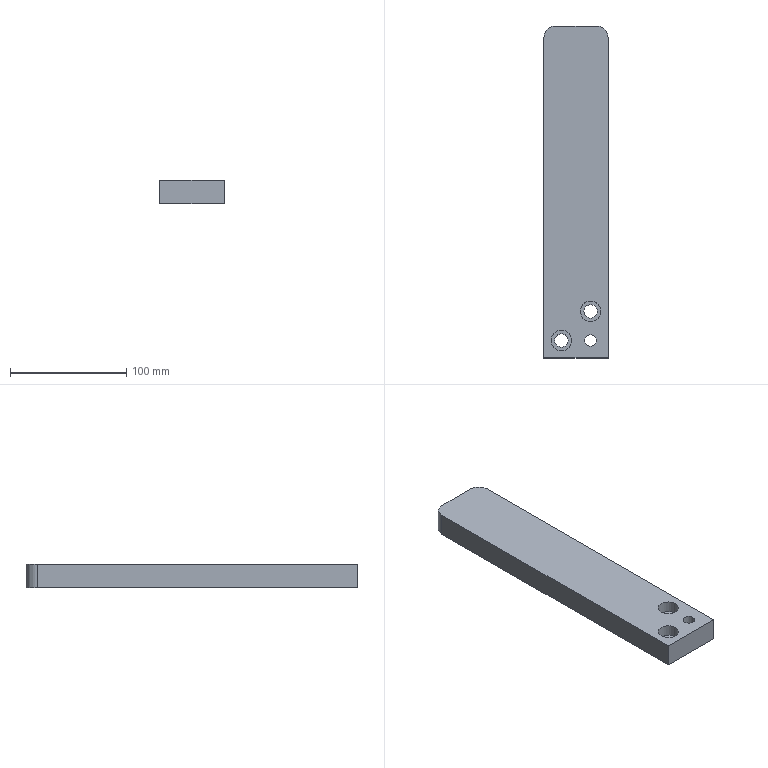Part | NX | features solid 2 | 1 solid | 15 faces | box 55 x 285 x 20 mm | volume 304183 mm3 | plane 8 | cylinder 7 | commonest cylinder face diameters 11.5 x2 17.5 x2 20 x2 10 x1
STEP:
#1=CARTESIAN_POINT('',(-295.,25.,-20.));
#2=VERTEX_POINT('',#1);
#3=CARTESIAN_POINT('',(-295.,25.,-40.));
#4=VERTEX_POINT('',#3);
#5=CARTESIAN_POINT('',(-295.,25.,-20.));
#6=DIRECTION('',(0.,0.,-1.));
#7=VECTOR('',#6,1000.);
#8=LINE('',#5,#7);
#9=EDGE_CURVE('',#2,#4,#8,.T.);
#10=ORIENTED_EDGE('',*,*,#9,.T.);
#11=CARTESIAN_POINT('',(-240.,25.,-40.));
#12=VERTEX_POINT('',#11);
#13=CARTESIAN_POINT('',(-290.,25.,-40.));
#14=DIRECTION('',(-1.,0.,0.));
#15=VECTOR('',#14,1000.);
#16=LINE('',#13,#15);
#17=EDGE_CURVE('',#4,#12,#16,.F.);
#18=ORIENTED_EDGE('',*,*,#17,.T.);
#19=CARTESIAN_POINT('',(-240.,25.,-20.));
#20=VERTEX_POINT('',#19);
#21=CARTESIAN_POINT('',(-240.,25.,-20.));
#22=DIRECTION('',(0.,0.,1.));
#23=VECTOR('',#22,1000.);
#24=LINE('',#21,#23);
#25=EDGE_CURVE('',#20,#12,#24,.F.);
#26=ORIENTED_EDGE('',*,*,#25,.F.);
#27=CARTESIAN_POINT('',(-290.,25.,-20.));
#28=DIRECTION('',(-1.,0.,0.));
#29=VECTOR('',#28,1000.);
#30=LINE('',#27,#29);
#31=EDGE_CURVE('',#2,#20,#30,.F.);
#32=ORIENTED_EDGE('',*,*,#31,.F.);
#33=EDGE_LOOP('',(#10,#18,#26,#32));
#34=FACE_BOUND('',#33,.T.);
#35=CARTESIAN_POINT('',(-290.,25.,-20.));
#36=DIRECTION('',(0.,1.,0.));
#37=DIRECTION('',(1.,0.,0.));
#38=AXIS2_PLACEMENT_3D('',#35,#36,#37);
#39=PLANE('',#38);
#40=ADVANCED_FACE('',(#34),#39,.F.);
#41=CARTESIAN_POINT('',(-250.,40.,-40.));
#42=VERTEX_POINT('',#41);
#43=CARTESIAN_POINT('',(-255.,40.,-40.));
#44=DIRECTION('',(0.,0.,1.));
#45=DIRECTION('',(1.,0.,0.));
#46=AXIS2_PLACEMENT_3D('',#43,#44,#45);
#47=CIRCLE('',#46,5.);
#48=EDGE_CURVE('',#42,#42,#47,.T.);
#49=ORIENTED_EDGE('',*,*,#48,.T.);
#50=EDGE_LOOP('',(#49));
#51=FACE_BOUND('',#50,.T.);
#52=CARTESIAN_POINT('',(-249.25,65.,-40.));
#53=VERTEX_POINT('',#52);
#54=CARTESIAN_POINT('',(-255.,65.,-40.));
#55=DIRECTION('',(0.,0.,1.));
#56=DIRECTION('',(1.,0.,0.));
#57=AXIS2_PLACEMENT_3D('',#54,#55,#56);
#58=CIRCLE('',#57,5.75);
#59=EDGE_CURVE('',#53,#53,#58,.T.);
#60=ORIENTED_EDGE('',*,*,#59,.T.);
#61=EDGE_LOOP('',(#60));
#62=FACE_BOUND('',#61,.T.);
#63=CARTESIAN_POINT('',(-274.25,40.,-40.));
#64=VERTEX_POINT('',#63);
#65=CARTESIAN_POINT('',(-280.,40.,-40.));
#66=DIRECTION('',(0.,0.,1.));
#67=DIRECTION('',(1.,0.,0.));
#68=AXIS2_PLACEMENT_3D('',#65,#66,#67);
#69=CIRCLE('',#68,5.75);
#70=EDGE_CURVE('',#64,#64,#69,.T.);
#71=ORIENTED_EDGE('',*,*,#70,.T.);
#72=EDGE_LOOP('',(#71));
#73=FACE_BOUND('',#72,.T.);
#74=CARTESIAN_POINT('',(-285.,310.,-40.));
#75=VERTEX_POINT('',#74);
#76=CARTESIAN_POINT('',(-250.,310.,-40.));
#77=VERTEX_POINT('',#76);
#78=CARTESIAN_POINT('',(-290.,310.,-40.));
#79=DIRECTION('',(1.,0.,0.));
#80=VECTOR('',#79,1000.);
#81=LINE('',#78,#80);
#82=EDGE_CURVE('',#75,#77,#81,.T.);
#83=ORIENTED_EDGE('',*,*,#82,.T.);
#84=CARTESIAN_POINT('',(-240.,300.,-40.));
#85=VERTEX_POINT('',#84);
#86=CARTESIAN_POINT('',(-250.,300.,-40.));
#87=DIRECTION('',(0.,0.,1.));
#88=DIRECTION('',(1.,0.,0.));
#89=AXIS2_PLACEMENT_3D('',#86,#87,#88);
#90=CIRCLE('',#89,10.);
#91=EDGE_CURVE('',#77,#85,#90,.F.);
#92=ORIENTED_EDGE('',*,*,#91,.T.);
#93=CARTESIAN_POINT('',(-240.,120.,-40.));
#94=DIRECTION('',(0.,-1.,0.));
#95=VECTOR('',#94,1000.);
#96=LINE('',#93,#95);
#97=EDGE_CURVE('',#85,#12,#96,.T.);
#98=ORIENTED_EDGE('',*,*,#97,.T.);
#99=ORIENTED_EDGE('',*,*,#17,.F.);
#100=CARTESIAN_POINT('',(-295.,300.,-40.));
#101=VERTEX_POINT('',#100);
#102=CARTESIAN_POINT('',(-295.,120.,-40.));
#103=DIRECTION('',(0.,1.,0.));
#104=VECTOR('',#103,1000.);
#105=LINE('',#102,#104);
#106=EDGE_CURVE('',#101,#4,#105,.F.);
#107=ORIENTED_EDGE('',*,*,#106,.F.);
#108=CARTESIAN_POINT('',(-285.,300.,-40.));
#109=DIRECTION('',(0.,0.,1.));
#110=DIRECTION('',(1.,0.,0.));
#111=AXIS2_PLACEMENT_3D('',#108,#109,#110);
#112=CIRCLE('',#111,10.);
#113=EDGE_CURVE('',#101,#75,#112,.F.);
#114=ORIENTED_EDGE('',*,*,#113,.T.);
#115=EDGE_LOOP('',(#83,#92,#98,#99,#107,#114));
#116=FACE_BOUND('',#115,.T.);
#117=CARTESIAN_POINT('',(-290.,120.,-40.));
#118=DIRECTION('',(0.,0.,1.));
#119=DIRECTION('',(-1.,0.,0.));
#120=AXIS2_PLACEMENT_3D('',#117,#118,#119);
#121=PLANE('',#120);
#122=ADVANCED_FACE('',(#51,#62,#73,#116),#121,.F.);
#123=CARTESIAN_POINT('',(-260.,40.,-20.));
#124=VERTEX_POINT('',#123);
#125=CARTESIAN_POINT('',(-255.,40.,-20.));
#126=DIRECTION('',(0.,0.,-1.));
#127=DIRECTION('',(-1.,0.,0.));
#128=AXIS2_PLACEMENT_3D('',#125,#126,#127);
#129=CIRCLE('',#128,5.);
#130=EDGE_CURVE('',#124,#124,#129,.T.);
#131=ORIENTED_EDGE('',*,*,#130,.T.);
#132=EDGE_LOOP('',(#131));
#133=FACE_BOUND('',#132,.T.);
#134=CARTESIAN_POINT('',(-263.75,65.,-20.));
#135=VERTEX_POINT('',#134);
#136=CARTESIAN_POINT('',(-255.,65.,-20.));
#137=DIRECTION('',(0.,0.,-1.));
#138=DIRECTION('',(-1.,0.,0.));
#139=AXIS2_PLACEMENT_3D('',#136,#137,#138);
#140=CIRCLE('',#139,8.75);
#141=EDGE_CURVE('',#135,#135,#140,.T.);
#142=ORIENTED_EDGE('',*,*,#141,.T.);
#143=EDGE_LOOP('',(#142));
#144=FACE_BOUND('',#143,.T.);
#145=CARTESIAN_POINT('',(-288.75,40.,-20.));
#146=VERTEX_POINT('',#145);
#147=CARTESIAN_POINT('',(-280.,40.,-20.));
#148=DIRECTION('',(0.,0.,-1.));
#149=DIRECTION('',(-1.,0.,0.));
#150=AXIS2_PLACEMENT_3D('',#147,#148,#149);
#151=CIRCLE('',#150,8.75);
#152=EDGE_CURVE('',#146,#146,#151,.T.);
#153=ORIENTED_EDGE('',*,*,#152,.T.);
#154=EDGE_LOOP('',(#153));
#155=FACE_BOUND('',#154,.T.);
#156=CARTESIAN_POINT('',(-240.,300.,-20.));
#157=VERTEX_POINT('',#156);
#158=CARTESIAN_POINT('',(-240.,120.,-20.));
#159=DIRECTION('',(0.,-1.,0.));
#160=VECTOR('',#159,1000.);
#161=LINE('',#158,#160);
#162=EDGE_CURVE('',#157,#20,#161,.T.);
#163=ORIENTED_EDGE('',*,*,#162,.F.);
#164=CARTESIAN_POINT('',(-250.,310.,-20.));
#165=VERTEX_POINT('',#164);
#166=CARTESIAN_POINT('',(-250.,300.,-20.));
#167=DIRECTION('',(0.,0.,1.));
#168=DIRECTION('',(1.,0.,0.));
#169=AXIS2_PLACEMENT_3D('',#166,#167,#168);
#170=CIRCLE('',#169,10.);
#171=EDGE_CURVE('',#157,#165,#170,.T.);
#172=ORIENTED_EDGE('',*,*,#171,.T.);
#173=CARTESIAN_POINT('',(-285.,310.,-20.));
#174=VERTEX_POINT('',#173);
#175=CARTESIAN_POINT('',(-290.,310.,-20.));
#176=DIRECTION('',(1.,0.,0.));
#177=VECTOR('',#176,1000.);
#178=LINE('',#175,#177);
#179=EDGE_CURVE('',#174,#165,#178,.T.);
#180=ORIENTED_EDGE('',*,*,#179,.F.);
#181=CARTESIAN_POINT('',(-295.,300.,-20.));
#182=VERTEX_POINT('',#181);
#183=CARTESIAN_POINT('',(-285.,300.,-20.));
#184=DIRECTION('',(0.,0.,1.));
#185=DIRECTION('',(1.,0.,0.));
#186=AXIS2_PLACEMENT_3D('',#183,#184,#185);
#187=CIRCLE('',#186,10.);
#188=EDGE_CURVE('',#174,#182,#187,.T.);
#189=ORIENTED_EDGE('',*,*,#188,.T.);
#190=CARTESIAN_POINT('',(-295.,120.,-20.));
#191=DIRECTION('',(0.,1.,0.));
#192=VECTOR('',#191,1000.);
#193=LINE('',#190,#192);
#194=EDGE_CURVE('',#182,#2,#193,.F.);
#195=ORIENTED_EDGE('',*,*,#194,.T.);
#196=ORIENTED_EDGE('',*,*,#31,.T.);
#197=EDGE_LOOP('',(#163,#172,#180,#189,#195,#196));
#198=FACE_BOUND('',#197,.T.);
#199=CARTESIAN_POINT('',(-290.,120.,-20.));
#200=DIRECTION('',(0.,0.,1.));
#201=DIRECTION('',(-1.,0.,0.));
#202=AXIS2_PLACEMENT_3D('',#199,#200,#201);
#203=PLANE('',#202);
#204=ADVANCED_FACE('',(#133,#144,#155,#198),#203,.T.);
#205=ORIENTED_EDGE('',*,*,#97,.F.);
#206=CARTESIAN_POINT('',(-240.,300.,-20.));
#207=DIRECTION('',(0.,0.,-1.));
#208=VECTOR('',#207,1000.);
#209=LINE('',#206,#208);
#210=EDGE_CURVE('',#85,#157,#209,.F.);
#211=ORIENTED_EDGE('',*,*,#210,.T.);
#212=ORIENTED_EDGE('',*,*,#162,.T.);
#213=ORIENTED_EDGE('',*,*,#25,.T.);
#214=EDGE_LOOP('',(#205,#211,#212,#213));
#215=FACE_BOUND('',#214,.T.);
#216=CARTESIAN_POINT('',(-240.,120.,-20.));
#217=DIRECTION('',(1.,0.,0.));
#218=DIRECTION('',(0.,-1.,0.));
#219=AXIS2_PLACEMENT_3D('',#216,#217,#218);
#220=PLANE('',#219);
#221=ADVANCED_FACE('',(#215),#220,.T.);
#222=ORIENTED_EDGE('',*,*,#194,.F.);
#223=CARTESIAN_POINT('',(-295.,300.,-20.));
#224=DIRECTION('',(0.,0.,1.));
#225=VECTOR('',#224,1000.);
#226=LINE('',#223,#225);
#227=EDGE_CURVE('',#182,#101,#226,.F.);
#228=ORIENTED_EDGE('',*,*,#227,.T.);
#229=ORIENTED_EDGE('',*,*,#106,.T.);
#230=ORIENTED_EDGE('',*,*,#9,.F.);
#231=EDGE_LOOP('',(#222,#228,#229,#230));
#232=FACE_BOUND('',#231,.T.);
#233=CARTESIAN_POINT('',(-295.,120.,-20.));
#234=DIRECTION('',(1.,0.,0.));
#235=DIRECTION('',(0.,-1.,0.));
#236=AXIS2_PLACEMENT_3D('',#233,#234,#235);
#237=PLANE('',#236);
#238=ADVANCED_FACE('',(#232),#237,.F.);
#239=ORIENTED_EDGE('',*,*,#179,.T.);
#240=CARTESIAN_POINT('',(-250.,310.,15.));
#241=DIRECTION('',(0.,0.,-1.));
#242=VECTOR('',#241,1000.);
#243=LINE('',#240,#242);
#244=EDGE_CURVE('',#165,#77,#243,.T.);
#245=ORIENTED_EDGE('',*,*,#244,.T.);
#246=ORIENTED_EDGE('',*,*,#82,.F.);
#247=CARTESIAN_POINT('',(-285.,310.,15.));
#248=DIRECTION('',(0.,0.,-1.));
#249=VECTOR('',#248,1000.);
#250=LINE('',#247,#249);
#251=EDGE_CURVE('',#75,#174,#250,.F.);
#252=ORIENTED_EDGE('',*,*,#251,.T.);
#253=EDGE_LOOP('',(#239,#245,#246,#252));
#254=FACE_BOUND('',#253,.T.);
#255=CARTESIAN_POINT('',(40.,310.,15.));
#256=DIRECTION('',(0.,1.,0.));
#257=DIRECTION('',(0.,0.,1.));
#258=AXIS2_PLACEMENT_3D('',#255,#256,#257);
#259=PLANE('',#258);
#260=ADVANCED_FACE('',(#254),#259,.T.);
#261=CARTESIAN_POINT('',(-274.25,40.,-30.));
#262=VERTEX_POINT('',#261);
#263=CARTESIAN_POINT('',(-280.,40.,-30.));
#264=DIRECTION('',(0.,0.,1.));
#265=DIRECTION('',(1.,0.,0.));
#266=AXIS2_PLACEMENT_3D('',#263,#264,#265);
#267=CIRCLE('',#266,5.75);
#268=EDGE_CURVE('',#262,#262,#267,.F.);
#269=ORIENTED_EDGE('',*,*,#268,.F.);
#270=EDGE_LOOP('',(#269));
#271=FACE_BOUND('',#270,.T.);
#272=ORIENTED_EDGE('',*,*,#70,.F.);
#273=EDGE_LOOP('',(#272));
#274=FACE_BOUND('',#273,.T.);
#275=CARTESIAN_POINT('',(-280.,40.,-115.));
#276=DIRECTION('',(0.,0.,-1.));
#277=DIRECTION('',(-1.,0.,0.));
#278=AXIS2_PLACEMENT_3D('',#275,#276,#277);
#279=CYLINDRICAL_SURFACE('',#278,5.75);
#280=ADVANCED_FACE('',(#271,#274),#279,.F.);
#281=ORIENTED_EDGE('',*,*,#268,.T.);
#282=EDGE_LOOP('',(#281));
#283=FACE_BOUND('',#282,.T.);
#284=CARTESIAN_POINT('',(-271.25,40.,-30.));
#285=VERTEX_POINT('',#284);
#286=CARTESIAN_POINT('',(-280.,40.,-30.));
#287=DIRECTION('',(0.,0.,1.));
#288=DIRECTION('',(1.,0.,0.));
#289=AXIS2_PLACEMENT_3D('',#286,#287,#288);
#290=CIRCLE('',#289,8.75);
#291=EDGE_CURVE('',#285,#285,#290,.F.);
#292=ORIENTED_EDGE('',*,*,#291,.F.);
#293=EDGE_LOOP('',(#292));
#294=FACE_BOUND('',#293,.T.);
#295=CARTESIAN_POINT('',(-280.,40.,-30.));
#296=DIRECTION('',(0.,0.,-1.));
#297=DIRECTION('',(-1.,0.,0.));
#298=AXIS2_PLACEMENT_3D('',#295,#296,#297);
#299=PLANE('',#298);
#300=ADVANCED_FACE('',(#283,#294),#299,.F.);
#301=ORIENTED_EDGE('',*,*,#291,.T.);
#302=EDGE_LOOP('',(#301));
#303=FACE_BOUND('',#302,.T.);
#304=ORIENTED_EDGE('',*,*,#152,.F.);
#305=EDGE_LOOP('',(#304));
#306=FACE_BOUND('',#305,.T.);
#307=CARTESIAN_POINT('',(-280.,40.,-15.));
#308=DIRECTION('',(0.,0.,-1.));
#309=DIRECTION('',(-1.,0.,0.));
#310=AXIS2_PLACEMENT_3D('',#307,#308,#309);
#311=CYLINDRICAL_SURFACE('',#310,8.75);
#312=ADVANCED_FACE('',(#303,#306),#311,.F.);
#313=CARTESIAN_POINT('',(-249.25,65.,-30.));
#314=VERTEX_POINT('',#313);
#315=CARTESIAN_POINT('',(-255.,65.,-30.));
#316=DIRECTION('',(0.,0.,1.));
#317=DIRECTION('',(1.,0.,0.));
#318=AXIS2_PLACEMENT_3D('',#315,#316,#317);
#319=CIRCLE('',#318,5.75);
#320=EDGE_CURVE('',#314,#314,#319,.F.);
#321=ORIENTED_EDGE('',*,*,#320,.F.);
#322=EDGE_LOOP('',(#321));
#323=FACE_BOUND('',#322,.T.);
#324=ORIENTED_EDGE('',*,*,#59,.F.);
#325=EDGE_LOOP('',(#324));
#326=FACE_BOUND('',#325,.T.);
#327=CARTESIAN_POINT('',(-255.,65.,-115.));
#328=DIRECTION('',(0.,0.,-1.));
#329=DIRECTION('',(-1.,0.,0.));
#330=AXIS2_PLACEMENT_3D('',#327,#328,#329);
#331=CYLINDRICAL_SURFACE('',#330,5.75);
#332=ADVANCED_FACE('',(#323,#326),#331,.F.);
#333=ORIENTED_EDGE('',*,*,#320,.T.);
#334=EDGE_LOOP('',(#333));
#335=FACE_BOUND('',#334,.T.);
#336=CARTESIAN_POINT('',(-246.25,65.,-30.));
#337=VERTEX_POINT('',#336);
#338=CARTESIAN_POINT('',(-255.,65.,-30.));
#339=DIRECTION('',(0.,0.,1.));
#340=DIRECTION('',(1.,0.,0.));
#341=AXIS2_PLACEMENT_3D('',#338,#339,#340);
#342=CIRCLE('',#341,8.75);
#343=EDGE_CURVE('',#337,#337,#342,.F.);
#344=ORIENTED_EDGE('',*,*,#343,.F.);
#345=EDGE_LOOP('',(#344));
#346=FACE_BOUND('',#345,.T.);
#347=CARTESIAN_POINT('',(-255.,65.,-30.));
#348=DIRECTION('',(0.,0.,-1.));
#349=DIRECTION('',(-1.,0.,0.));
#350=AXIS2_PLACEMENT_3D('',#347,#348,#349);
#351=PLANE('',#350);
#352=ADVANCED_FACE('',(#335,#346),#351,.F.);
#353=ORIENTED_EDGE('',*,*,#343,.T.);
#354=EDGE_LOOP('',(#353));
#355=FACE_BOUND('',#354,.T.);
#356=ORIENTED_EDGE('',*,*,#141,.F.);
#357=EDGE_LOOP('',(#356));
#358=FACE_BOUND('',#357,.T.);
#359=CARTESIAN_POINT('',(-255.,65.,-15.));
#360=DIRECTION('',(0.,0.,-1.));
#361=DIRECTION('',(-1.,0.,0.));
#362=AXIS2_PLACEMENT_3D('',#359,#360,#361);
#363=CYLINDRICAL_SURFACE('',#362,8.75);
#364=ADVANCED_FACE('',(#355,#358),#363,.F.);
#365=ORIENTED_EDGE('',*,*,#130,.F.);
#366=EDGE_LOOP('',(#365));
#367=FACE_BOUND('',#366,.T.);
#368=ORIENTED_EDGE('',*,*,#48,.F.);
#369=EDGE_LOOP('',(#368));
#370=FACE_BOUND('',#369,.T.);
#371=CARTESIAN_POINT('',(-255.,40.,-15.));
#372=DIRECTION('',(0.,0.,-1.));
#373=DIRECTION('',(-1.,0.,0.));
#374=AXIS2_PLACEMENT_3D('',#371,#372,#373);
#375=CYLINDRICAL_SURFACE('',#374,5.);
#376=ADVANCED_FACE('',(#367,#370),#375,.F.);
#377=ORIENTED_EDGE('',*,*,#113,.F.);
#378=ORIENTED_EDGE('',*,*,#227,.F.);
#379=ORIENTED_EDGE('',*,*,#188,.F.);
#380=ORIENTED_EDGE('',*,*,#251,.F.);
#381=EDGE_LOOP('',(#377,#378,#379,#380));
#382=FACE_BOUND('',#381,.T.);
#383=CARTESIAN_POINT('',(-285.,300.,15.));
#384=DIRECTION('',(0.,0.,-1.));
#385=DIRECTION('',(-1.,0.,0.));
#386=AXIS2_PLACEMENT_3D('',#383,#384,#385);
#387=CYLINDRICAL_SURFACE('',#386,10.);
#388=ADVANCED_FACE('',(#382),#387,.T.);
#389=ORIENTED_EDGE('',*,*,#171,.F.);
#390=ORIENTED_EDGE('',*,*,#210,.F.);
#391=ORIENTED_EDGE('',*,*,#91,.F.);
#392=ORIENTED_EDGE('',*,*,#244,.F.);
#393=EDGE_LOOP('',(#389,#390,#391,#392));
#394=FACE_BOUND('',#393,.T.);
#395=CARTESIAN_POINT('',(-250.,300.,15.));
#396=DIRECTION('',(0.,0.,-1.));
#397=DIRECTION('',(-1.,0.,0.));
#398=AXIS2_PLACEMENT_3D('',#395,#396,#397);
#399=CYLINDRICAL_SURFACE('',#398,10.);
#400=ADVANCED_FACE('',(#394),#399,.T.);
#401=CLOSED_SHELL('',(#40,#122,#204,#221,#238,#260,#280,#300,#312,#332,#352,#364,#376,#388,#400));
#402=MANIFOLD_SOLID_BREP('',#401);
#403=(LENGTH_UNIT()NAMED_UNIT(*)SI_UNIT(.MILLI.,.METRE.));
#404=UNCERTAINTY_MEASURE_WITH_UNIT(LENGTH_MEASURE(0.00001),#403,'','');
#405=(NAMED_UNIT(*)PLANE_ANGLE_UNIT()SI_UNIT($,.RADIAN.));
#406=(NAMED_UNIT(*)SI_UNIT($,.STERADIAN.)SOLID_ANGLE_UNIT());
#407=(GEOMETRIC_REPRESENTATION_CONTEXT(3)GLOBAL_UNCERTAINTY_ASSIGNED_CONTEXT((#404))GLOBAL_UNIT_ASSIGNED_CONTEXT((#403,#405,#406))REPRESENTATION_CONTEXT('',''));
#408=ADVANCED_BREP_SHAPE_REPRESENTATION('',(#402),#407);